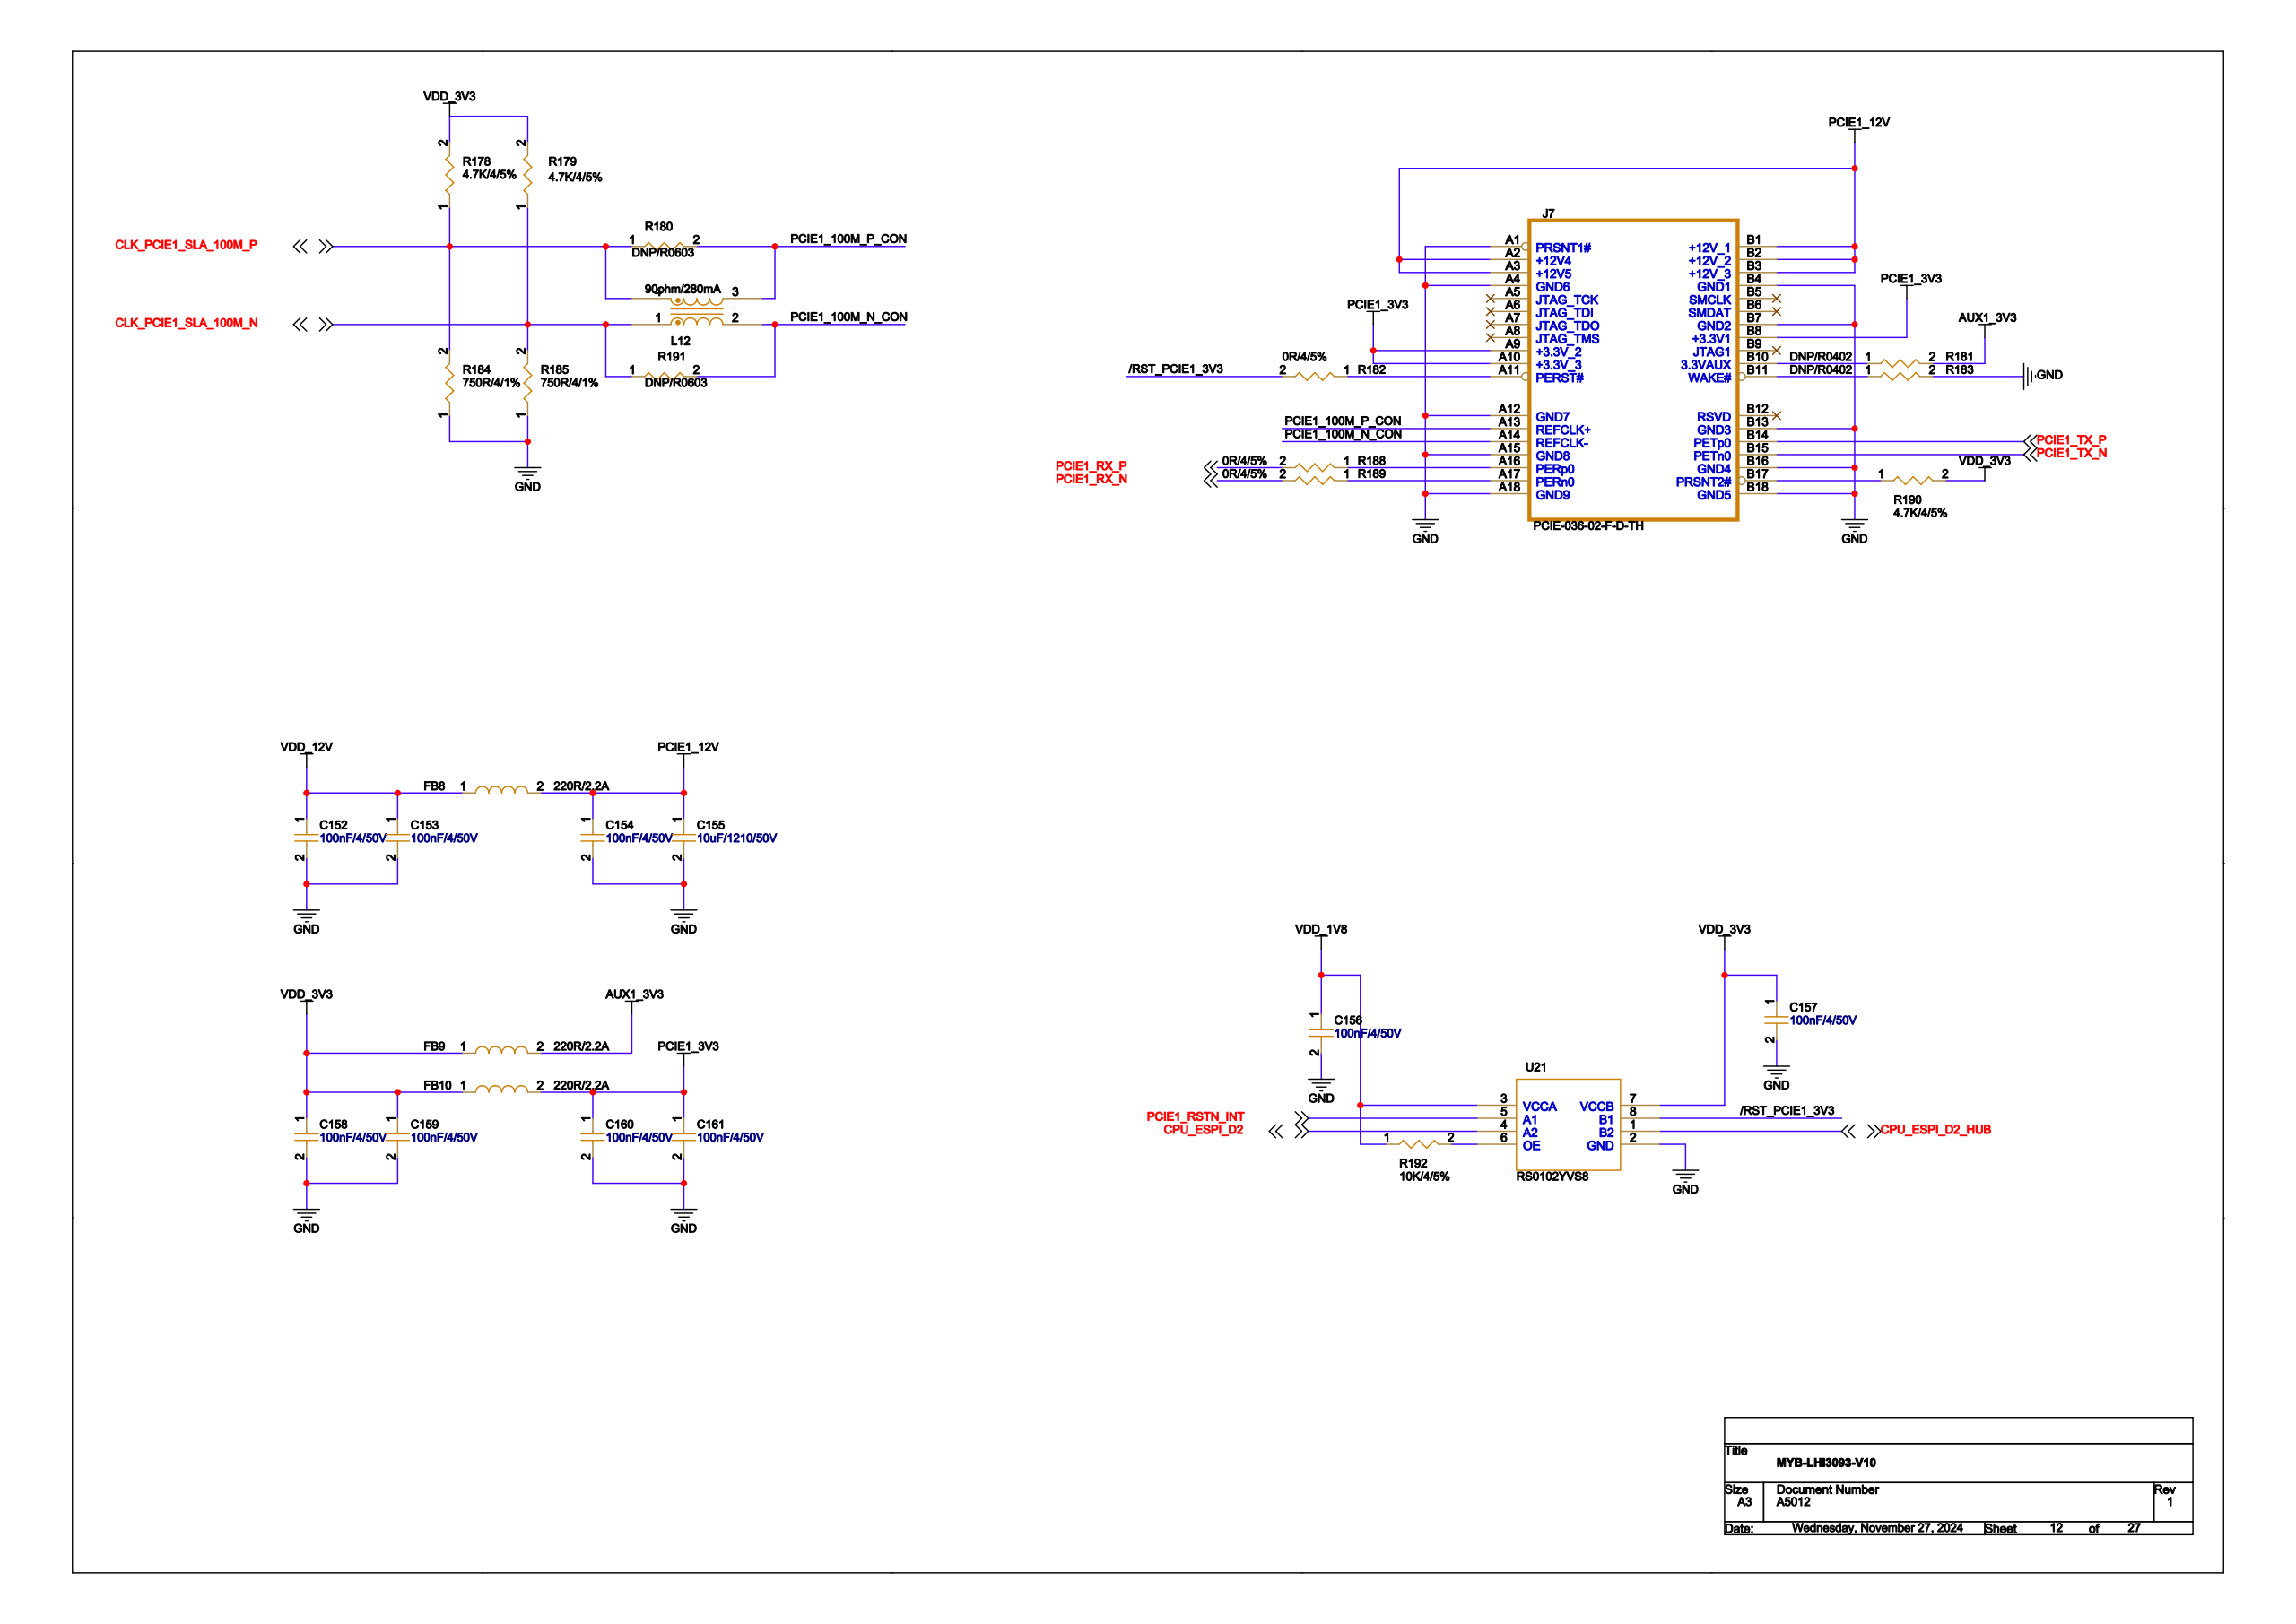Circuit board | Cadence Allegro | 1159 parts | 708 nets | one sheet of the schematic
Parts on this sheet (reference | value | footprint):
C152 | 100nF/4/50V | C0402
C153 | 100nF/4/50V | C0402
C154 | 100nF/4/50V | C0402
C155 | 10uF/1210/50V | C1210
C156 | 100nF/4/50V | C0402
C157 | 100nF/4/50V | C0402
C158 | 100nF/4/50V | C0402
C159 | 100nF/4/50V | C0402
C160 | 100nF/4/50V | C0402
C161 | 100nF/4/50V | C0402
FB8 | 220R/2.2A | FB0603
FB9 | 220R/2.2A | FB0603
FB10 | 220R/2.2A | FB0603
J7 | PCIE-036-02-F-D-TH | CONN-PCIE-036-02-F-D-TH
L12 | 90ohm/280mA | INDCM-SDCW2012
R178 | 4.7K/4/5% | R0402
R179 | 4.7K/4/5% | R0402
R180 | DNP/R0603 | R0603
R181 | DNP/R0402 | R0402
R182 | 0R/4/5% | R0402
R183 | DNP/R0402 | R0402
R184 | 750R/4/1% | R0402
R185 | 750R/4/1% | R0402
R188 | 0R/4/5% | R0402
R189 | 0R/4/5% | R0402
R190 | 4.7K/4/5% | R0402
R191 | DNP/R0603 | R0603
R192 | 10K/4/5% | R0402
U21 | RS0102YVS8 | VSSOP8
Nets of these parts (net: part-pin ...):
GND: C152-2 C153-2 C154-2 C155-2 C156-2 C157-2 C158-2 C159-2 C160-2 C161-2 R183-2 R184-1 R185-1 U21-2 J7-A1 J7-A4 J7-A12 J7-A15 J7-A18 J7-B4 J7-B7 J7-B13 J7-B16 J7-B18
VDD_12V: C152-1 C153-1 FB8-1
VDD_3V3: C157-1 C158-1 C159-1 FB9-1 FB10-1 R178-2 R179-2 R190-2 U21-7
PCIE1_12V: C154-1 C155-1 FB8-2 J7-A2 J7-A3 J7-B1 J7-B2 J7-B3
VDD_1V8: C156-1 R192-1 U21-3
PCIE1_3V3: C160-1 C161-1 FB10-2 J7-A9 J7-A10 J7-B8
PCIE1_RSTN_INT: U21-5
CLK_PCIE1_SLA_100M_N: L12-1 R179-1 R185-2 R191-1
CLK_PCIE1_SLA_100M_P: L12-4 R178-1 R180-1 R184-2
AUX1_3V3: FB9-2 R181-2
N14890678: R181-1 J7-B10
N14891347: R189-1 J7-A17
N14891343: R188-1 J7-A16
N14891481: R182-1 J7-A11
PCIE1_TX_N: J7-B15
PCIE1_TX_P: J7-B14
N14890416: R190-1 J7-B17
PCIE1_100M_P_CON: L12-3 R180-2 J7-A13
PCIE1_100M_N_CON: L12-2 R191-2 J7-A14
N14890682: R183-1 J7-B11
CPU_ESPI_D2_HUB: U21-1
/RST_PCIE1_3V3: R182-2 U21-8
PCIE1_RX_P: R188-2
PCIE1_RX_N: R189-2
N14889369: R192-2 U21-6
CPU_ESPI_D2: U21-4